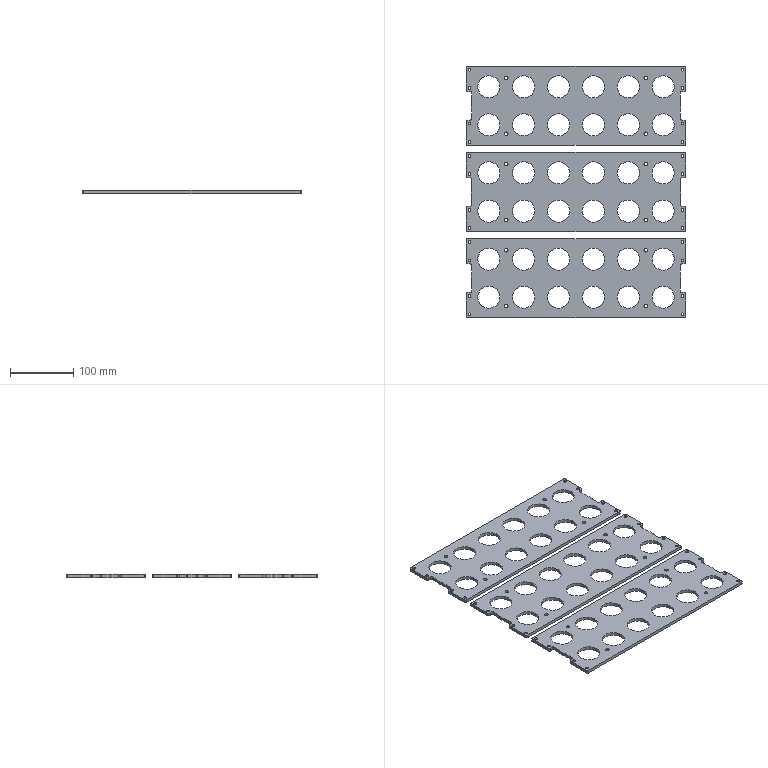CAM job | NX | 3-axis milling, drilling | part box 346 x 397 x 5 mm | stock box 351 x 402 x 5 mm
Tools:
number,name,description,diameter,corner_radius,flute_length,length,flutes
4,D4,平底铣刀-粗,4.0,0.0,25.0,75.0,2
9,D10,平底铣刀-粗,10.0,0.0,35.0,75.0,2
17,D2-J,平底铣刀-精,2.0,0.0,50.0,75.0,2
19,D3-J,平底铣刀-精,3.0,0.0,50.0,75.0,2
11,D4-J,平底铣刀-精,4.0,0.0,50.0,75.0,2
7,D6-J,平底铣刀-精,6.0,0.0,25.0,75.0,2
2,D6_CHAMFERTOOL,倒角刀,6.0,0.0,3.0,25.0,2
11,ZT4.5,钻头,4.5,0.0,35.0,50.0,2
18,ZT5.5,钻头,5.5,0.0,35.0,50.0,2
Operations:
program,operation,operation_type,tool,method,geometry_group,spindle_rpm,surface_speed,feed_per_tooth,feed_cut,feed_plunge,cut_length_mm,path_length_mm,cut_time_min,machine_time_min
A,SPOTDRILL,Operation,D6_CHAMFERTOOL,METHOD,W-A,3000.0,56.549,0.0333,200.0,0.0,180.0,3210.405,0.9,1.203
A,DRILLHOLES,Operation,ZT4.5,METHOD,W-A,2800.0,39.584,0.0214,120.0,0.0,136.8,1464.953,1.14,1.273
A,DRILLHOLES_2,Operation,ZT5.5,METHOD,W-A,2600.0,44.925,0.0231,120.0,0.0,68.4,1147.878,0.57,0.6779
A,FLOORWALL_SPIRALROUGH-MID_COPY,VolumeBased25DMillingOperation,D10,LAYERED_ROUGH-DEPTHK-STEPG,W-A,8000.0,251.327,0.125,2000.0,100.0,25982.227,31056.417,12.991,13.498
A,PROFILE_ROUGH_2,VolumeBased25DMillingOperation,D10,METHOD,W-A,6000.0,188.0,0.25,4000.0,80.0,35745.22,36341.421,8.936,8.996
A,ZSTOCK0.5_FLOORWALLOFFSET0.1_RAMPFINISH-MID_COPY,VolumeBased25DMillingOperation,D6-J,SIDEFINISH-DEPTHK-STEPG,W-A,8000.0,150.792,0.0625,1000.0,100.0,4439.86,8859.372,4.44,4.882
A,FLOORWALL_LAYERROUGH-MID_COPY,VolumeBased25DMillingOperation,D4,LAYERED_ROUGH-DEPTHK-STEPG,W-A,8000.0,100.528,0.125,2000.0,100.0,823.431,1151.587,0.4117,0.4445
A,ZLEVELSPIRALCLIMB_COPY,ZLevelMilling,D4-J,ZLEVELCLIMB-DEPTHK-STEPG,W-A,7000.0,87.965,0.1429,2000.0,100.0,39083.456,41675.487,19.542,19.801
A,FLOORWALL_FINISHFLOOR-MID_COPY,VolumeBased25DMillingOperation,D2-J,FINISH_STEPDEPTHOFF,W-A,8000.0,100.528,0.05,800.0,100.0,770.157,1099.117,0.9627,0.9956
A,FLOORWALL_FINISHWALL-MID-SELFLOOR_COPY,VolumeBased25DMillingOperation,D2-J,SIDEFINISH-DEPTHK-STEPG,W-A,8000.0,100.528,0.05,800.0,100.0,198.17,548.898,0.2477,0.2828
A,ZLEVELSMOOTHCORNER_D2REF6_COPY,ZLevelMilling,D2-J,LAYERED_FINISH-DEPTHK-STEPG,W-A,8000.0,50.266,0.0938,1500.0,100.0,4922.663,7755.755,3.282,3.565
A,FLOORWALL_SPIRALFINISH-MID_COPY_COPY,VolumeBased25DMillingOperation,D3-J,SPIRALFINISH-DEPTHK-STEPG,W-A,8000.0,75.398,0.0312,500.0,100.0,2207.097,6322.125,4.414,4.826
A,BODYONLY,SurfaceContour,D6_CHAMFERTOOL,METHOD,W-A,6000.0,113.0,0.125,1200.0,100.0,6946.024,11671.183,5.788,6.261
A,DRILL_CHAMFER_1,Operation,D6_CHAMFERTOOL,METHOD,W-A,5000.0,94.248,0.015,150.0,0.0,184.8,1609.767,1.232,1.375
A,MILL_CHAMFER_1,PlanarMilling,D6_CHAMFERTOOL,METHOD,W-A,6000.0,113.097,0.05,600.0,100.0,213.535,1895.007,0.3559,0.524
A,PROFILE_SEMIFINISH_2,VolumeBased25DMillingOperation,D6-J,METHOD,W-A,6000.0,113.0,0.0833,1000.0,100.0,2964.813,3739.848,2.965,3.042
A,PROFILE_FINISH_2,VolumeBased25DMillingOperation,D6-J,METHOD,W-A,6000.0,113.0,0.0833,1000.0,100.0,2964.213,3740.918,2.964,3.042